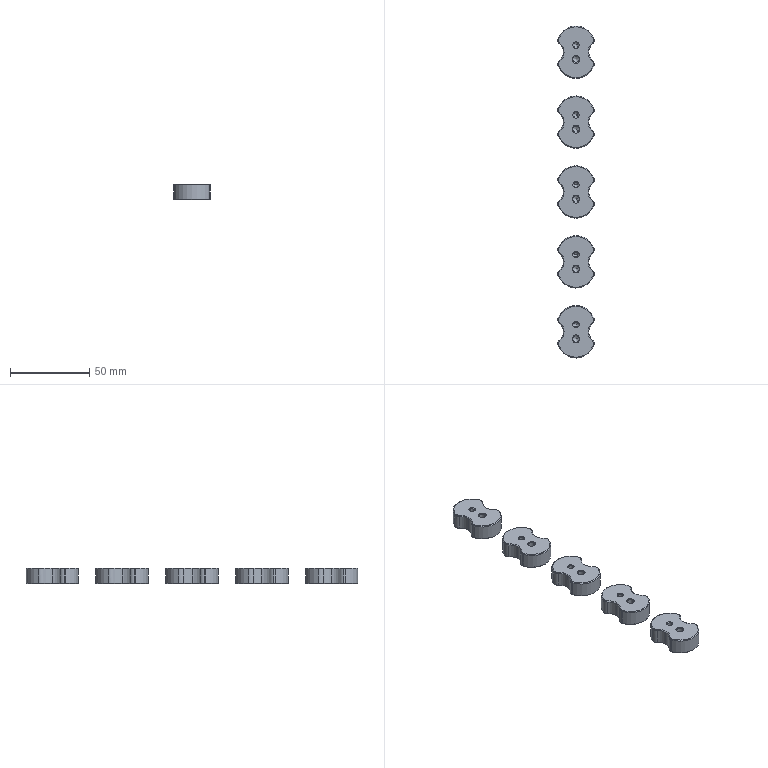NC program | NX | posted with a generic post | part box 22.923 x 209 x 10 mm
Whole program:
N10 G17 G21 G94 G90
(FLOOR_WALL_COPY , TOOL : D80)
N12 T19 M6
N14 G54
N16 G17 G0 G90 X-149.5 Y0. S6500 M3
N18 G43 Z30. H19
N20 Z7.5
N22 G94 G1 Z4.5 F1500.
N24 X-144.5
N26 X144.5
N28 X149.5
N30 Z7.5
N32 G0 Z30.
N34 X-149.5
N36 Z7.
N38 G1 Z4.
N40 X-144.5
N42 X144.5
N44 X149.5
N46 Z7.
N48 G0 Z30.
N50 X-149.5
N52 Z6.5
N54 G1 Z3.5
N56 X-144.5
N58 X144.5
N60 X149.5
N62 Z6.5
N64 G0 Z30.
N66 X-149.5
N68 Z6.
N70 G1 Z3.
N72 X-144.5
N74 X144.5
N76 X149.5
N78 Z6.
N80 G0 Z30.
N82 X-149.5
N84 Z5.5
N86 G1 Z2.5
N88 X-144.5
N90 X144.5
N92 X149.5
N94 Z5.5
N96 G0 Z30.
N98 X-149.5
N100 Z5.
N102 G1 Z2.
N104 X-144.5
N106 X144.5
N108 X149.5
N110 Z5.
N112 G0 Z30.
N114 X-149.5
N116 Z4.5
N118 G1 Z1.5
N120 X-144.5
N122 X144.5
N124 X149.5
N126 Z4.5
N128 G0 Z30.
N130 X-149.5
N132 Z4.
N134 G1 Z1.
N136 X-144.5
N138 X144.5
N140 X149.5
N142 Z4.
N144 G0 Z30.
N146 X-149.5
N148 Z3.5
N150 G1 Z0.5
N152 X-144.5
N154 X144.5
N156 X149.5
N158 Z3.5
N160 G0 Z30.
N162 X-149.5
N164 Z3.
N166 G1 Z0.
N168 X-144.5
N170 X144.5
N172 X149.5
N174 Z3.
N176 G0 Z30.
N178 M5
(PLANAR_MILL_COPY_COPY_COPY_COPY_COPY , TOOL : D6A45)
N180 T01 M6
N182 G54
N184 G17 G0 G90 X-106. Y-0.866 S9500 M3
N186 G43 Z30. H1
N188 Z0.
N190 G94 G1 Z-1.5 F1250.
N192 G3 X-105.5 Y0. R1.
N194 G2 X-96.929 Y12.222 R13.
N196 X-92.54 Y11.077 R4.
N198 G3 X-83.46 Y11.077 R6.
N200 G2 X-79.071 Y12.222 R4.
N202 X-79.071 Y-12.222 R13.
N204 X-83.46 Y-11.077 R4.
N206 G3 X-92.54 Y-11.077 R6.
N208 G2 X-96.929 Y-12.222 R4.
N210 X-105.5 Y0. R13.
N212 G3 X-106. Y0.866 R1.
N214 G1 Z0.
N216 G0 Z30.
N218 X-62. Y-0.866
N220 Z0.
N222 G1 Z-1.5
N224 G3 X-61.5 Y0. R1.
N226 G2 X-52.929 Y12.222 R13.
N228 X-48.54 Y11.077 R4.
N230 G3 X-39.46 Y11.077 R6.
N232 G2 X-35.071 Y12.222 R4.
N234 X-35.071 Y-12.222 R13.
N236 X-39.46 Y-11.077 R4.
N238 G3 X-48.54 Y-11.077 R6.
N240 G2 X-52.929 Y-12.222 R4.
N242 X-61.5 Y0. R13.
N244 G3 X-62. Y0.866 R1.
N246 G1 Z0.
N248 G0 Z30.
N250 X-18. Y-0.866
N252 Z0.
N254 G1 Z-1.5
N256 G3 X-17.5 Y0. R1.
N258 G2 X-8.929 Y12.222 R13.
N260 X-4.54 Y11.077 R4.
N262 G3 X4.54 Y11.077 R6.
N264 G2 X8.929 Y12.222 R4.
N266 X8.929 Y-12.222 R13.
N268 X4.54 Y-11.077 R4.
N270 G3 X-4.54 Y-11.077 R6.
N272 G2 X-8.929 Y-12.222 R4.
N274 X-17.5 Y0. R13.
N276 G3 X-18. Y0.866 R1.
N278 G1 Z0.
N280 G0 Z30.
N282 X26. Y-0.866
N284 Z0.
N286 G1 Z-1.5
N288 G3 X26.5 Y0. R1.
N290 G2 X35.071 Y12.222 R13.
N292 X39.46 Y11.077 R4.
N294 G3 X48.54 Y11.077 R6.
N296 G2 X52.929 Y12.222 R4.
N298 X52.929 Y-12.222 R13.
N300 X48.54 Y-11.077 R4.
N302 G3 X39.46 Y-11.077 R6.
N304 G2 X35.071 Y-12.222 R4.
N306 X26.5 Y0. R13.
N308 G3 X26. Y0.866 R1.
N310 G1 Z0.
N312 G0 Z30.
N314 X106.
N316 Z0.
N318 G1 Z-1.5
N320 G3 X105.5 Y0. R1.
N322 G2 X96.929 Y-12.222 R13.
N324 X92.54 Y-11.077 R4.
N326 G3 X83.46 Y-11.077 R6.
N328 G2 X79.071 Y-12.222 R4.
N330 X79.071 Y12.222 R13.
N332 X83.46 Y11.077 R4.
N334 G3 X92.54 Y11.077 R6.
N336 G2 X96.929 Y12.222 R4.
N338 X105.5 Y0. R13.
N340 G3 X106. Y-0.866 R1.
N342 G1 Z0.
N344 G0 Z30.
N346 M5
N348 M2